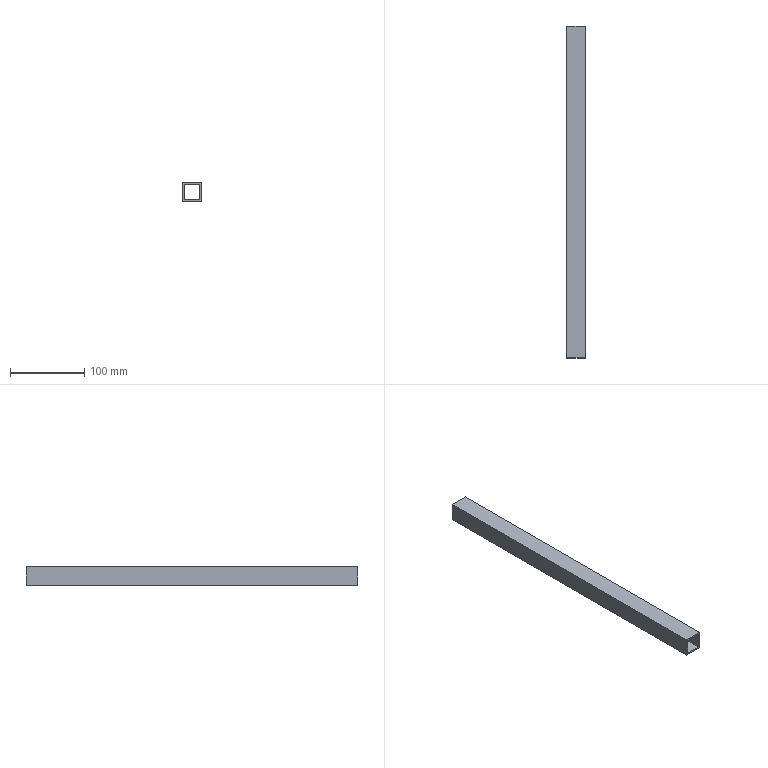Part | NX | features solid 2 | 1 solid | 10 faces | box 25 x 448 x 25 mm | volume 82432 mm3 | plane 10
STEP:
#1=CARTESIAN_POINT('',(348.5,221.,-75.));
#2=VERTEX_POINT('',#1);
#3=CARTESIAN_POINT('',(348.5,-227.,-75.));
#4=VERTEX_POINT('',#3);
#5=CARTESIAN_POINT('',(348.5,-147.,-75.));
#6=DIRECTION('',(0.,-1.,0.));
#7=VECTOR('',#6,1000.);
#8=LINE('',#5,#7);
#9=EDGE_CURVE('',#2,#4,#8,.T.);
#10=ORIENTED_EDGE('',*,*,#9,.F.);
#11=CARTESIAN_POINT('',(373.5,221.,-75.));
#12=VERTEX_POINT('',#11);
#13=CARTESIAN_POINT('',(578.,221.,-75.));
#14=DIRECTION('',(-1.,0.,0.));
#15=VECTOR('',#14,1000.);
#16=LINE('',#13,#15);
#17=EDGE_CURVE('',#12,#2,#16,.T.);
#18=ORIENTED_EDGE('',*,*,#17,.F.);
#19=CARTESIAN_POINT('',(373.5,-227.,-75.));
#20=VERTEX_POINT('',#19);
#21=CARTESIAN_POINT('',(373.5,-147.,-75.));
#22=DIRECTION('',(0.,-1.,0.));
#23=VECTOR('',#22,1000.);
#24=LINE('',#21,#23);
#25=EDGE_CURVE('',#12,#20,#24,.T.);
#26=ORIENTED_EDGE('',*,*,#25,.T.);
#27=CARTESIAN_POINT('',(346.,-227.,-75.));
#28=DIRECTION('',(1.,0.,0.));
#29=VECTOR('',#28,1000.);
#30=LINE('',#27,#29);
#31=EDGE_CURVE('',#4,#20,#30,.T.);
#32=ORIENTED_EDGE('',*,*,#31,.F.);
#33=EDGE_LOOP('',(#10,#18,#26,#32));
#34=FACE_BOUND('',#33,.T.);
#35=CARTESIAN_POINT('',(346.,-147.,-75.));
#36=DIRECTION('',(0.,0.,-1.));
#37=DIRECTION('',(1.,0.,0.));
#38=AXIS2_PLACEMENT_3D('',#35,#36,#37);
#39=PLANE('',#38);
#40=ADVANCED_FACE('',(#34),#39,.T.);
#41=CARTESIAN_POINT('',(348.5,221.,-50.));
#42=VERTEX_POINT('',#41);
#43=CARTESIAN_POINT('',(348.5,-227.,-50.));
#44=VERTEX_POINT('',#43);
#45=CARTESIAN_POINT('',(348.5,-147.,-50.));
#46=DIRECTION('',(0.,-1.,0.));
#47=VECTOR('',#46,1000.);
#48=LINE('',#45,#47);
#49=EDGE_CURVE('',#42,#44,#48,.T.);
#50=ORIENTED_EDGE('',*,*,#49,.F.);
#51=CARTESIAN_POINT('',(348.5,221.,-296.5));
#52=DIRECTION('',(0.,0.,1.));
#53=VECTOR('',#52,1000.);
#54=LINE('',#51,#53);
#55=EDGE_CURVE('',#2,#42,#54,.T.);
#56=ORIENTED_EDGE('',*,*,#55,.F.);
#57=ORIENTED_EDGE('',*,*,#9,.T.);
#58=CARTESIAN_POINT('',(348.5,-227.,-47.5));
#59=DIRECTION('',(0.,0.,-1.));
#60=VECTOR('',#59,1000.);
#61=LINE('',#58,#60);
#62=EDGE_CURVE('',#44,#4,#61,.T.);
#63=ORIENTED_EDGE('',*,*,#62,.F.);
#64=EDGE_LOOP('',(#50,#56,#57,#63));
#65=FACE_BOUND('',#64,.T.);
#66=CARTESIAN_POINT('',(348.5,-147.,-47.5));
#67=DIRECTION('',(-1.,0.,0.));
#68=DIRECTION('',(0.,0.,-1.));
#69=AXIS2_PLACEMENT_3D('',#66,#67,#68);
#70=PLANE('',#69);
#71=ADVANCED_FACE('',(#65),#70,.T.);
#72=CARTESIAN_POINT('',(373.5,221.,-50.));
#73=VERTEX_POINT('',#72);
#74=CARTESIAN_POINT('',(373.5,-227.,-50.));
#75=VERTEX_POINT('',#74);
#76=CARTESIAN_POINT('',(373.5,-147.,-50.));
#77=DIRECTION('',(0.,-1.,0.));
#78=VECTOR('',#77,1000.);
#79=LINE('',#76,#78);
#80=EDGE_CURVE('',#73,#75,#79,.T.);
#81=ORIENTED_EDGE('',*,*,#80,.F.);
#82=CARTESIAN_POINT('',(578.,221.,-50.));
#83=DIRECTION('',(1.,0.,0.));
#84=VECTOR('',#83,1000.);
#85=LINE('',#82,#84);
#86=EDGE_CURVE('',#42,#73,#85,.T.);
#87=ORIENTED_EDGE('',*,*,#86,.F.);
#88=ORIENTED_EDGE('',*,*,#49,.T.);
#89=CARTESIAN_POINT('',(376.,-227.,-50.));
#90=DIRECTION('',(-1.,0.,0.));
#91=VECTOR('',#90,1000.);
#92=LINE('',#89,#91);
#93=EDGE_CURVE('',#75,#44,#92,.T.);
#94=ORIENTED_EDGE('',*,*,#93,.F.);
#95=EDGE_LOOP('',(#81,#87,#88,#94));
#96=FACE_BOUND('',#95,.T.);
#97=CARTESIAN_POINT('',(376.,-147.,-50.));
#98=DIRECTION('',(0.,0.,1.));
#99=DIRECTION('',(-1.,0.,0.));
#100=AXIS2_PLACEMENT_3D('',#97,#98,#99);
#101=PLANE('',#100);
#102=ADVANCED_FACE('',(#96),#101,.T.);
#103=ORIENTED_EDGE('',*,*,#25,.F.);
#104=CARTESIAN_POINT('',(373.5,221.,-296.5));
#105=DIRECTION('',(0.,0.,-1.));
#106=VECTOR('',#105,1000.);
#107=LINE('',#104,#106);
#108=EDGE_CURVE('',#73,#12,#107,.T.);
#109=ORIENTED_EDGE('',*,*,#108,.F.);
#110=ORIENTED_EDGE('',*,*,#80,.T.);
#111=CARTESIAN_POINT('',(373.5,-227.,-77.5));
#112=DIRECTION('',(0.,0.,1.));
#113=VECTOR('',#112,1000.);
#114=LINE('',#111,#113);
#115=EDGE_CURVE('',#20,#75,#114,.T.);
#116=ORIENTED_EDGE('',*,*,#115,.F.);
#117=EDGE_LOOP('',(#103,#109,#110,#116));
#118=FACE_BOUND('',#117,.T.);
#119=CARTESIAN_POINT('',(373.5,-147.,-77.5));
#120=DIRECTION('',(1.,0.,0.));
#121=DIRECTION('',(0.,0.,1.));
#122=AXIS2_PLACEMENT_3D('',#119,#120,#121);
#123=PLANE('',#122);
#124=ADVANCED_FACE('',(#118),#123,.T.);
#125=CARTESIAN_POINT('',(371.5,221.,-73.));
#126=VERTEX_POINT('',#125);
#127=CARTESIAN_POINT('',(371.5,-227.,-73.));
#128=VERTEX_POINT('',#127);
#129=CARTESIAN_POINT('',(371.5,-147.,-73.));
#130=DIRECTION('',(0.,-1.,0.));
#131=VECTOR('',#130,1000.);
#132=LINE('',#129,#131);
#133=EDGE_CURVE('',#126,#128,#132,.T.);
#134=ORIENTED_EDGE('',*,*,#133,.F.);
#135=CARTESIAN_POINT('',(350.5,221.,-73.));
#136=VERTEX_POINT('',#135);
#137=CARTESIAN_POINT('',(578.,221.,-73.));
#138=DIRECTION('',(-1.,0.,0.));
#139=VECTOR('',#138,1000.);
#140=LINE('',#137,#139);
#141=EDGE_CURVE('',#126,#136,#140,.T.);
#142=ORIENTED_EDGE('',*,*,#141,.T.);
#143=CARTESIAN_POINT('',(350.5,-227.,-73.));
#144=VERTEX_POINT('',#143);
#145=CARTESIAN_POINT('',(350.5,-147.,-73.));
#146=DIRECTION('',(0.,-1.,0.));
#147=VECTOR('',#146,1000.);
#148=LINE('',#145,#147);
#149=EDGE_CURVE('',#136,#144,#148,.T.);
#150=ORIENTED_EDGE('',*,*,#149,.T.);
#151=CARTESIAN_POINT('',(346.,-227.,-73.));
#152=DIRECTION('',(1.,0.,0.));
#153=VECTOR('',#152,1000.);
#154=LINE('',#151,#153);
#155=EDGE_CURVE('',#144,#128,#154,.T.);
#156=ORIENTED_EDGE('',*,*,#155,.T.);
#157=EDGE_LOOP('',(#134,#142,#150,#156));
#158=FACE_BOUND('',#157,.T.);
#159=CARTESIAN_POINT('',(346.,-147.,-73.));
#160=DIRECTION('',(0.,0.,-1.));
#161=DIRECTION('',(1.,0.,0.));
#162=AXIS2_PLACEMENT_3D('',#159,#160,#161);
#163=PLANE('',#162);
#164=ADVANCED_FACE('',(#158),#163,.F.);
#165=ORIENTED_EDGE('',*,*,#149,.F.);
#166=CARTESIAN_POINT('',(350.5,221.,-52.));
#167=VERTEX_POINT('',#166);
#168=CARTESIAN_POINT('',(350.5,221.,-296.5));
#169=DIRECTION('',(0.,0.,1.));
#170=VECTOR('',#169,1000.);
#171=LINE('',#168,#170);
#172=EDGE_CURVE('',#136,#167,#171,.T.);
#173=ORIENTED_EDGE('',*,*,#172,.T.);
#174=CARTESIAN_POINT('',(350.5,-227.,-52.));
#175=VERTEX_POINT('',#174);
#176=CARTESIAN_POINT('',(350.5,-147.,-52.));
#177=DIRECTION('',(0.,-1.,0.));
#178=VECTOR('',#177,1000.);
#179=LINE('',#176,#178);
#180=EDGE_CURVE('',#167,#175,#179,.T.);
#181=ORIENTED_EDGE('',*,*,#180,.T.);
#182=CARTESIAN_POINT('',(350.5,-227.,-47.5));
#183=DIRECTION('',(0.,0.,-1.));
#184=VECTOR('',#183,1000.);
#185=LINE('',#182,#184);
#186=EDGE_CURVE('',#175,#144,#185,.T.);
#187=ORIENTED_EDGE('',*,*,#186,.T.);
#188=EDGE_LOOP('',(#165,#173,#181,#187));
#189=FACE_BOUND('',#188,.T.);
#190=CARTESIAN_POINT('',(350.5,-147.,-47.5));
#191=DIRECTION('',(-1.,0.,0.));
#192=DIRECTION('',(0.,0.,-1.));
#193=AXIS2_PLACEMENT_3D('',#190,#191,#192);
#194=PLANE('',#193);
#195=ADVANCED_FACE('',(#189),#194,.F.);
#196=ORIENTED_EDGE('',*,*,#180,.F.);
#197=CARTESIAN_POINT('',(371.5,221.,-52.));
#198=VERTEX_POINT('',#197);
#199=CARTESIAN_POINT('',(578.,221.,-52.));
#200=DIRECTION('',(1.,0.,0.));
#201=VECTOR('',#200,1000.);
#202=LINE('',#199,#201);
#203=EDGE_CURVE('',#167,#198,#202,.T.);
#204=ORIENTED_EDGE('',*,*,#203,.T.);
#205=CARTESIAN_POINT('',(371.5,-227.,-52.));
#206=VERTEX_POINT('',#205);
#207=CARTESIAN_POINT('',(371.5,-147.,-52.));
#208=DIRECTION('',(0.,-1.,0.));
#209=VECTOR('',#208,1000.);
#210=LINE('',#207,#209);
#211=EDGE_CURVE('',#198,#206,#210,.T.);
#212=ORIENTED_EDGE('',*,*,#211,.T.);
#213=CARTESIAN_POINT('',(376.,-227.,-52.));
#214=DIRECTION('',(-1.,0.,0.));
#215=VECTOR('',#214,1000.);
#216=LINE('',#213,#215);
#217=EDGE_CURVE('',#206,#175,#216,.T.);
#218=ORIENTED_EDGE('',*,*,#217,.T.);
#219=EDGE_LOOP('',(#196,#204,#212,#218));
#220=FACE_BOUND('',#219,.T.);
#221=CARTESIAN_POINT('',(376.,-147.,-52.));
#222=DIRECTION('',(0.,0.,1.));
#223=DIRECTION('',(-1.,0.,0.));
#224=AXIS2_PLACEMENT_3D('',#221,#222,#223);
#225=PLANE('',#224);
#226=ADVANCED_FACE('',(#220),#225,.F.);
#227=ORIENTED_EDGE('',*,*,#211,.F.);
#228=CARTESIAN_POINT('',(371.5,221.,-296.5));
#229=DIRECTION('',(0.,0.,-1.));
#230=VECTOR('',#229,1000.);
#231=LINE('',#228,#230);
#232=EDGE_CURVE('',#198,#126,#231,.T.);
#233=ORIENTED_EDGE('',*,*,#232,.T.);
#234=ORIENTED_EDGE('',*,*,#133,.T.);
#235=CARTESIAN_POINT('',(371.5,-227.,-77.5));
#236=DIRECTION('',(0.,0.,1.));
#237=VECTOR('',#236,1000.);
#238=LINE('',#235,#237);
#239=EDGE_CURVE('',#128,#206,#238,.T.);
#240=ORIENTED_EDGE('',*,*,#239,.T.);
#241=EDGE_LOOP('',(#227,#233,#234,#240));
#242=FACE_BOUND('',#241,.T.);
#243=CARTESIAN_POINT('',(371.5,-147.,-77.5));
#244=DIRECTION('',(1.,0.,0.));
#245=DIRECTION('',(0.,0.,1.));
#246=AXIS2_PLACEMENT_3D('',#243,#244,#245);
#247=PLANE('',#246);
#248=ADVANCED_FACE('',(#242),#247,.F.);
#249=ORIENTED_EDGE('',*,*,#115,.T.);
#250=ORIENTED_EDGE('',*,*,#93,.T.);
#251=ORIENTED_EDGE('',*,*,#62,.T.);
#252=ORIENTED_EDGE('',*,*,#31,.T.);
#253=EDGE_LOOP('',(#249,#250,#251,#252));
#254=FACE_BOUND('',#253,.T.);
#255=ORIENTED_EDGE('',*,*,#155,.F.);
#256=ORIENTED_EDGE('',*,*,#186,.F.);
#257=ORIENTED_EDGE('',*,*,#217,.F.);
#258=ORIENTED_EDGE('',*,*,#239,.F.);
#259=EDGE_LOOP('',(#255,#256,#257,#258));
#260=FACE_BOUND('',#259,.T.);
#261=CARTESIAN_POINT('',(130.,-227.,-51.5));
#262=DIRECTION('',(0.,1.,0.));
#263=DIRECTION('',(0.,0.,1.));
#264=AXIS2_PLACEMENT_3D('',#261,#262,#263);
#265=PLANE('',#264);
#266=ADVANCED_FACE('',(#254,#260),#265,.F.);
#267=ORIENTED_EDGE('',*,*,#17,.T.);
#268=ORIENTED_EDGE('',*,*,#55,.T.);
#269=ORIENTED_EDGE('',*,*,#86,.T.);
#270=ORIENTED_EDGE('',*,*,#108,.T.);
#271=EDGE_LOOP('',(#267,#268,#269,#270));
#272=FACE_BOUND('',#271,.T.);
#273=ORIENTED_EDGE('',*,*,#232,.F.);
#274=ORIENTED_EDGE('',*,*,#203,.F.);
#275=ORIENTED_EDGE('',*,*,#172,.F.);
#276=ORIENTED_EDGE('',*,*,#141,.F.);
#277=EDGE_LOOP('',(#273,#274,#275,#276));
#278=FACE_BOUND('',#277,.T.);
#279=CARTESIAN_POINT('',(578.,221.,-296.5));
#280=DIRECTION('',(0.,1.,0.));
#281=DIRECTION('',(1.,0.,0.));
#282=AXIS2_PLACEMENT_3D('',#279,#280,#281);
#283=PLANE('',#282);
#284=ADVANCED_FACE('',(#272,#278),#283,.T.);
#285=CLOSED_SHELL('',(#40,#71,#102,#124,#164,#195,#226,#248,#266,#284));
#286=MANIFOLD_SOLID_BREP('',#285);
#287=(LENGTH_UNIT()NAMED_UNIT(*)SI_UNIT(.MILLI.,.METRE.));
#288=UNCERTAINTY_MEASURE_WITH_UNIT(LENGTH_MEASURE(0.00001),#287,'','');
#289=(NAMED_UNIT(*)PLANE_ANGLE_UNIT()SI_UNIT($,.RADIAN.));
#290=(NAMED_UNIT(*)SI_UNIT($,.STERADIAN.)SOLID_ANGLE_UNIT());
#291=(GEOMETRIC_REPRESENTATION_CONTEXT(3)GLOBAL_UNCERTAINTY_ASSIGNED_CONTEXT((#288))GLOBAL_UNIT_ASSIGNED_CONTEXT((#287,#289,#290))REPRESENTATION_CONTEXT('',''));
#292=ADVANCED_BREP_SHAPE_REPRESENTATION('',(#286),#291);